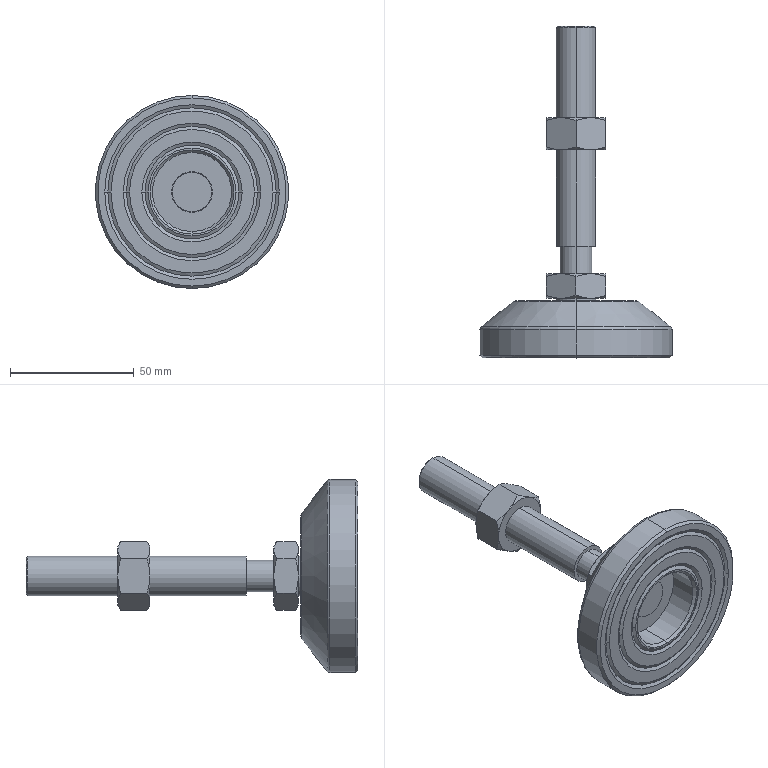Part | STEP file | 2 solids | 93 faces | box 78 x 134 x 78 mm | volume 111485 mm3 | cone 50 | plane 25 | cylinder 14 | torus 4 | commonest cylinder face diameters 16 x6 12.8 x2 16.5 x2 32 x2 78 x2